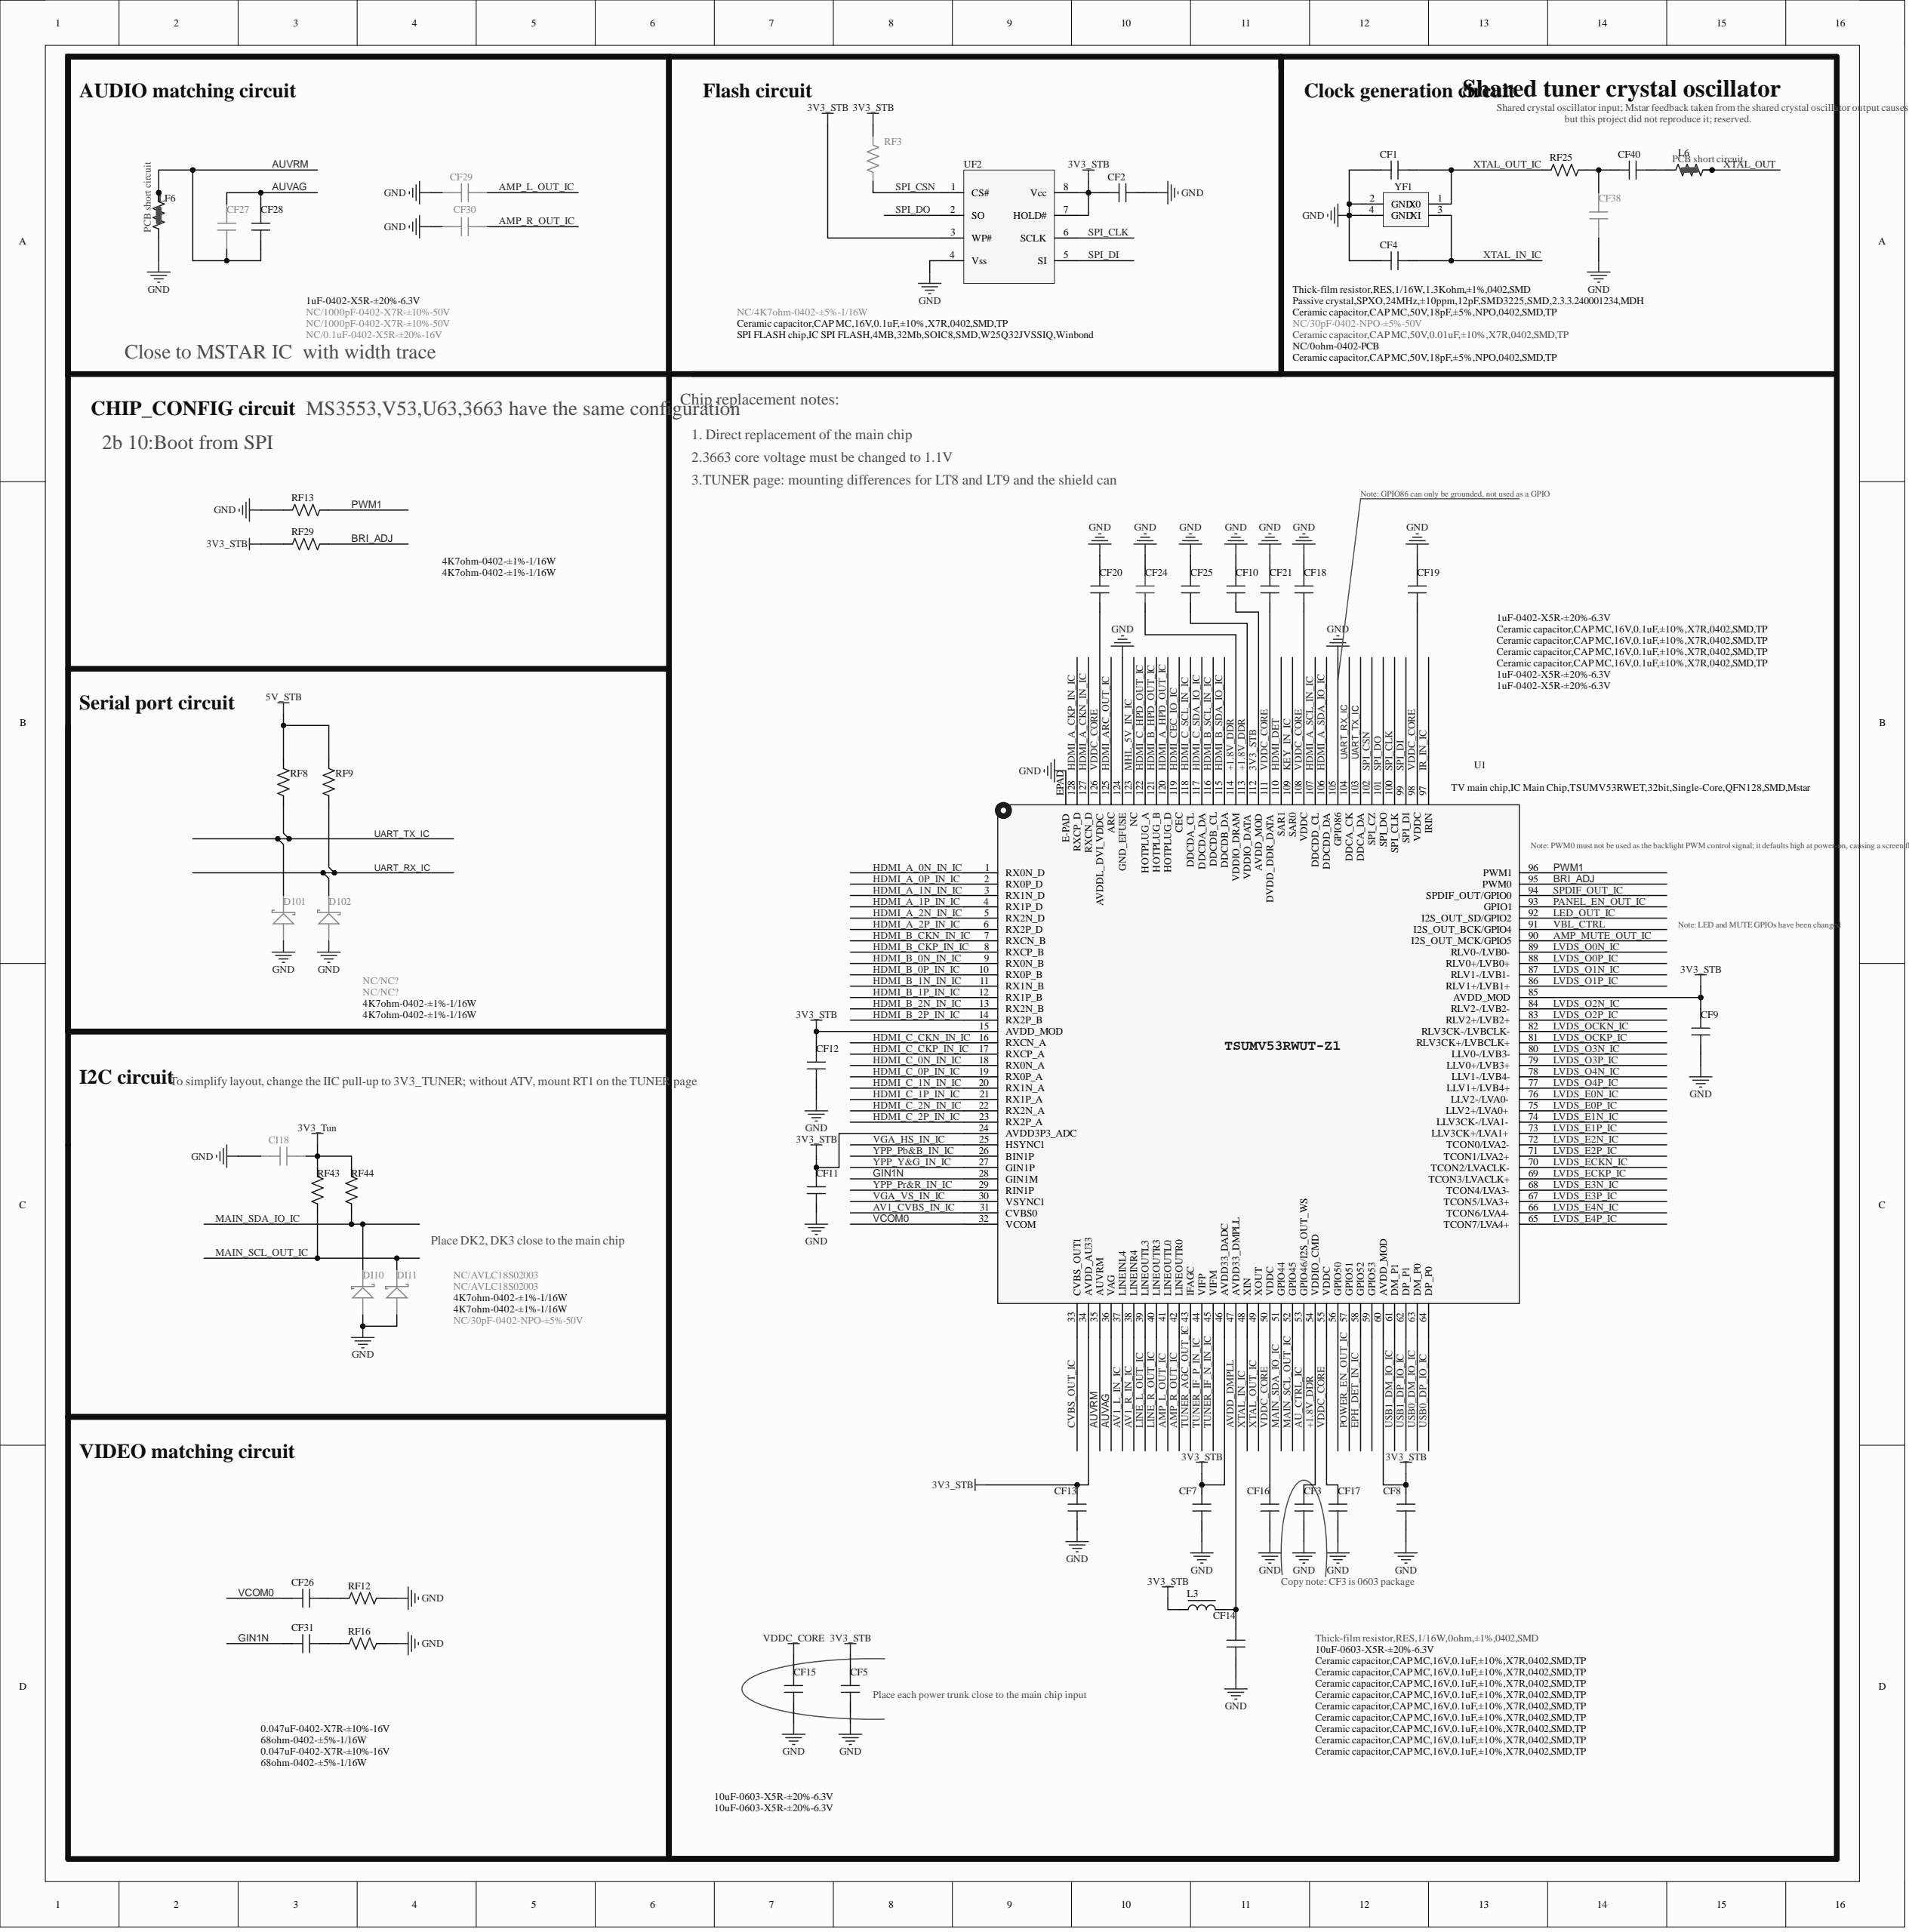Circuit board | Altium Designer | 527 parts | 243 nets | one sheet of the schematic
Parts on this sheet (reference | value | footprint):
CF1 | Ceramic capacitor,CAP MC,50V,18pF,±5%,NPO,0402,SMD,TP | C0402
CF2 | Ceramic capacitor,CAP MC,16V,0.1uF,±10%,X7R,0402,SMD,TP | C0402
CF3 | 10uF-0603-X5R-±20%-6.3V | C0603
CF4 | Ceramic capacitor,CAP MC,50V,18pF,±5%,NPO,0402,SMD,TP | C0402
CF5 | 10uF-0603-X5R-±20%-6.3V | C0603
CF7 | Ceramic capacitor,CAP MC,16V,0.1uF,±10%,X7R,0402,SMD,TP | C0402
CF8 | Ceramic capacitor,CAP MC,16V,0.1uF,±10%,X7R,0402,SMD,TP | C0402
CF9 | Ceramic capacitor,CAP MC,16V,0.1uF,±10%,X7R,0402,SMD,TP | C0402
CF10 | Ceramic capacitor,CAP MC,16V,0.1uF,±10%,X7R,0402,SMD,TP | C0402
CF11 | Ceramic capacitor,CAP MC,16V,0.1uF,±10%,X7R,0402,SMD,TP | C0402
CF12 | Ceramic capacitor,CAP MC,16V,0.1uF,±10%,X7R,0402,SMD,TP | C0402
CF13 | Ceramic capacitor,CAP MC,16V,0.1uF,±10%,X7R,0402,SMD,TP | C0402
CF14 | Ceramic capacitor,CAP MC,16V,0.1uF,±10%,X7R,0402,SMD,TP | C0402
CF15 | 10uF-0603-X5R-±20%-6.3V | C0603
CF16 | Ceramic capacitor,CAP MC,16V,0.1uF,±10%,X7R,0402,SMD,TP | C0402
CF17 | Ceramic capacitor,CAP MC,16V,0.1uF,±10%,X7R,0402,SMD,TP | C0402
CF18 | Ceramic capacitor,CAP MC,16V,0.1uF,±10%,X7R,0402,SMD,TP | C0402
CF19 | Ceramic capacitor,CAP MC,16V,0.1uF,±10%,X7R,0402,SMD,TP | C0402
CF20 | Ceramic capacitor,CAP MC,16V,0.1uF,±10%,X7R,0402,SMD,TP | C0402
CF21 | 1uF-0402-X5R-±20%-6.3V | C0402
CF24 | 1uF-0402-X5R-±20%-6.3V | C0402
CF25 | 1uF-0402-X5R-±20%-6.3V | C0402
CF26 | 0.047uF-0402-X7R-±10%-16V | C0402
CF27 | NC/0.1uF-0402-X5R-±20%-16V | C0402
CF28 | 1uF-0402-X5R-±20%-6.3V | C0402
CF29 | NC/1000pF-0402-X7R-±10%-50V | C0402
CF30 | NC/1000pF-0402-X7R-±10%-50V | C0402
CF31 | 0.047uF-0402-X7R-±10%-16V | C0402
CF38 | NC/30pF-0402-NPO-±5%-50V | C0402
CF40 | Ceramic capacitor,CAP MC,50V,0.01uF,±10%,X7R,0402,SMD,TP | C0402
CI18 | NC/30pF-0402-NPO-±5%-50V | C0402
D101 | NC/NC? | DIODE-S0402
D102 | NC/NC? | DIODE-S0402
DI10 | NC/AVLC18S02003 | DIODE-S0402
DI11 | NC/AVLC18S02003 | DIODE-S0402
L3 | Thick-film resistor,RES,1/16W,0ohm,±1%,0402,SMD | L0402
L6 | NC/0ohm-0402-PCB | R0402SC
LF6 | NC/0ohm-0402-PCB | R0402SC
RF3 | NC/4K7ohm-0402-±5%-1/16W | R0402
RF8 | 4K7ohm-0402-±1%-1/16W | R0402
RF9 | 4K7ohm-0402-±1%-1/16W | R0402
RF12 | 68ohm-0402-±5%-1/16W | R0402
RF13 | 4K7ohm-0402-±1%-1/16W | R0402
RF16 | 68ohm-0402-±5%-1/16W | R0402
RF25 | Thick-film resistor,RES,1/16W,1.3Kohm,±1%,0402,SMD | R0402
RF29 | 4K7ohm-0402-±1%-1/16W | R0402
RF43 | 4K7ohm-0402-±1%-1/16W | R0402
RF44 | 4K7ohm-0402-±1%-1/16W | R0402
U1 | TV main chip,IC Main Chip,TSUMV53RWET,32bit,Single-Core,QFN128,SMD,Mstar | QFN128/0.35-1
UF2 | SPI FLASH chip,IC SPI FLASH,4MB,32Mb,SOIC8,SMD,W25Q32JVSSIQ,Winbond | SOIC8
YF1 | Passive crystal,SPXO,24MHz,±10ppm,12pF,SMD3225,SMD,2.3.3.240001234,MDH | XTAL-S-3
Nets of these parts (net: part-pin ...):
YPP_Y&G_IN_IC: U1-27
YPP_Pr&R_IN_IC: U1-29
YPP_Pb&B_IN_IC: U1-26
XTAL_OUT_IC: CF1-2 RF25-2 YF1-1 U1-49
XTAL_OUT: L6-2 L6-3
XTAL_IN_IC: CF4-2 YF1-3 U1-48
VDDC_CORE: CF15-2 CF16-2 CF17-2 CF18-1 CF19-1 CF20-2 CF21-1 U1-50 U1-55 U1-98 U1-108 U1-111 U1-126
VCOM0: CF26-1 U1-32
USB0_DP_IO_IC: U1-64
USB0_DM_IO_IC: U1-63
UART_TX_IC: D101-K RF8-1 U1-103
UART_RX_IC: D102-K RF9-1 U1-104
TUNER_IF_P_IN_IC: U1-44
TUNER_IF_N_IN_IC: U1-45
SPI_DO: UF2-2 U1-101
SPI_DI: UF2-5 U1-99
SPI_CSN: RF3-1 UF2-1 U1-102
SPI_CLK: UF2-6 U1-100
SPDIF_OUT_IC: U1-94
PWM1: RF13-1 U1-96
POWER_EN_OUT_IC: U1-57
PANEL_EN_OUT_IC: U1-93
NetCF40_1: CF40-1 L6-1
NetCF38_2: CF38-2 CF40-2 RF25-1
NetCF31_2: CF31-2 RF16-1
NetCF26_2: CF26-2 RF12-1
MAIN_SDA_IO_IC: DI10-K RF44-2 U1-51
MAIN_SCL_OUT_IC: DI11-K RF43-2 U1-52
LVDS_OCKP_IC: U1-81
LVDS_OCKN_IC: U1-82
LVDS_O3P_IC: U1-79
LVDS_O3N_IC: U1-80
LVDS_O2P_IC: U1-83
LVDS_O2N_IC: U1-84
LVDS_O1P_IC: U1-86
LVDS_O1N_IC: U1-87
LVDS_O0P_IC: U1-88
LVDS_O0N_IC: U1-89
LVDS_ECKP_IC: U1-69
LVDS_ECKN_IC: U1-70
LVDS_E3P_IC: U1-67
LVDS_E3N_IC: U1-68
LVDS_E2P_IC: U1-71
LVDS_E2N_IC: U1-72
LVDS_E1P_IC: U1-73
LVDS_E1N_IC: U1-74
LVDS_E0P_IC: U1-75
LVDS_E0N_IC: U1-76
LINE_R_OUT_IC: U1-40
LINE_L_OUT_IC: U1-39
LED_OUT_IC: U1-92
KEY_IN_IC: U1-109
IR_IN_IC: U1-97
HDMI_DET: U1-110
HDMI_CEC_IO_IC: U1-119
HDMI_ARC_OUT_IC: U1-125
HDMI_A_SDA_IO_IC: U1-106
HDMI_A_SCL_IN_IC: U1-107
HDMI_A_HPD_OUT_IC: U1-120
HDMI_A_CKP_IN_IC: U1-128
HDMI_A_CKN_IN_IC: U1-127
HDMI_A_2P_IN_IC: U1-6
HDMI_A_2N_IN_IC: U1-5
HDMI_A_1P_IN_IC: U1-4
HDMI_A_1N_IN_IC: U1-3
HDMI_A_0P_IN_IC: U1-2
HDMI_A_0N_IN_IC: U1-1
GND: CF1-1 CF2-1 CF3-1 CF4-1 CF5-1 CF7-1 CF8-1 CF9-1 CF10-1 CF11-2 CF12-1 CF13-1 CF14-1 CF15-1 CF16-1 CF17-1 CF18-2 CF19-2 CF20-1 CF21-2 CF24-2 CF25-2 CF29-2 CF30-2 CF38-1 CI18-1 D101-A D102-A DI10-A DI11-A LF6-1 RF12-2 RF13-2 RF16-2 UF2-4 YF1-2 YF1-4 U1-105 U1-124 U1-EPAD
GIN1N: CF31-1 U1-28
EPH_DET_IN_IC: U1-58
CVBS_OUT_IC: U1-33
BRI_ADJ: RF29-1 U1-95
AVDD_DMPLL: CF14-2 L3-2 U1-47
AV1_R_IN_IC: U1-38
AV1_L_IN_IC: U1-37
AV1_CVBS_IN_IC: U1-31
AUVRM: CF27-1 CF28-1 LF6-2 LF6-3 U1-35
AUVAG: CF27-2 CF28-2 U1-36
AMP_R_OUT_IC: CF30-1 U1-42
AMP_MUTE_OUT_IC: U1-90
AMP_L_OUT_IC: CF29-1 U1-41
+1.8V_DDR: CF3-2 CF24-1 CF25-1 U1-54 U1-113 U1-114
5V_STB: RF8-2 RF9-2
3V3_Tun: CI18-2 RF43-1 RF44-1
3V3_STB: CF2-2 CF5-2 CF7-2 CF8-2 CF9-2 CF10-2 CF11-1 CF12-2 CF13-2 L3-1 RF3-2 RF29-2 UF2-3 UF2-7 UF2-8 U1-15 U1-24 U1-34 U1-46 U1-60 U1-85 U1-112